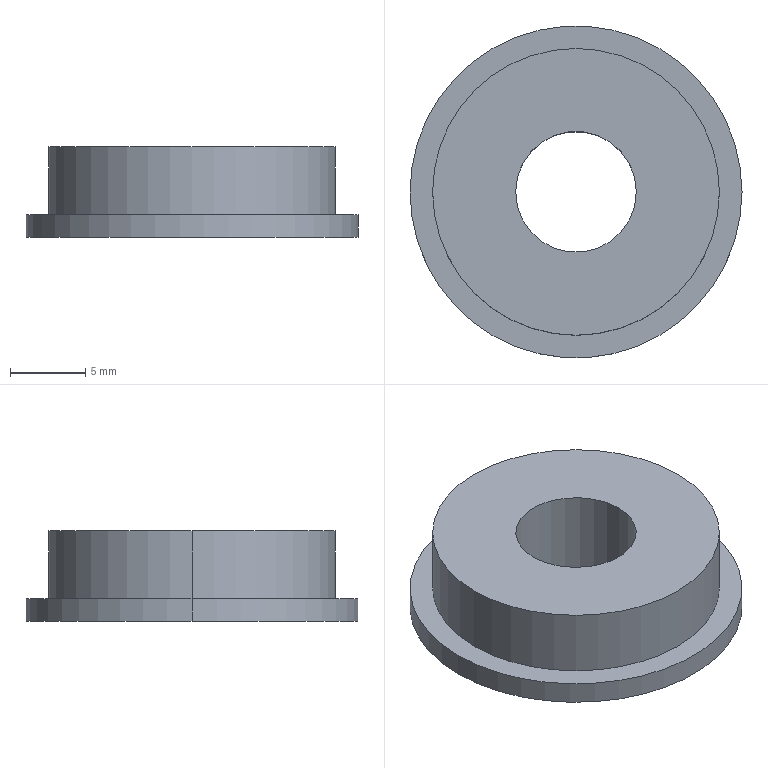Part | NX | 1 solid | 9 faces | box 22 x 22 x 6 mm | volume 1544 mm3 | cylinder 6 | plane 3 | commonest cylinder face diameters 8 x2 19 x2 22 x2
STEP:
#1=CARTESIAN_POINT('',(655.81,171.903,-33.25));
#2=VERTEX_POINT('',#1);
#3=CARTESIAN_POINT('',(633.81,171.903,-33.25));
#4=VERTEX_POINT('',#3);
#5=CARTESIAN_POINT('',(644.81,171.903,-33.25));
#6=DIRECTION('',(0.,0.,1.));
#7=DIRECTION('',(1.,0.,0.));
#8=AXIS2_PLACEMENT_3D('',#5,#6,#7);
#9=CIRCLE('',#8,11.);
#10=EDGE_CURVE('',#2,#4,#9,.T.);
#11=ORIENTED_EDGE('',*,*,#10,.T.);
#12=CARTESIAN_POINT('',(633.81,171.903,-31.75));
#13=VERTEX_POINT('',#12);
#14=CARTESIAN_POINT('',(633.81,171.903,-33.25));
#15=DIRECTION('',(0.,0.,1.));
#16=VECTOR('',#15,1000.);
#17=LINE('',#14,#16);
#18=EDGE_CURVE('',#4,#13,#17,.T.);
#19=ORIENTED_EDGE('',*,*,#18,.T.);
#20=CARTESIAN_POINT('',(655.81,171.903,-31.75));
#21=VERTEX_POINT('',#20);
#22=CARTESIAN_POINT('',(644.81,171.903,-31.75));
#23=DIRECTION('',(0.,0.,1.));
#24=DIRECTION('',(1.,0.,0.));
#25=AXIS2_PLACEMENT_3D('',#22,#23,#24);
#26=CIRCLE('',#25,11.);
#27=EDGE_CURVE('',#21,#13,#26,.T.);
#28=ORIENTED_EDGE('',*,*,#27,.F.);
#29=CARTESIAN_POINT('',(655.81,171.903,-33.25));
#30=DIRECTION('',(0.,0.,1.));
#31=VECTOR('',#30,1000.);
#32=LINE('',#29,#31);
#33=EDGE_CURVE('',#2,#21,#32,.T.);
#34=ORIENTED_EDGE('',*,*,#33,.F.);
#35=EDGE_LOOP('',(#11,#19,#28,#34));
#36=FACE_BOUND('',#35,.T.);
#37=CARTESIAN_POINT('',(644.81,171.903,-33.25));
#38=DIRECTION('',(0.,0.,1.));
#39=DIRECTION('',(1.,0.,0.));
#40=AXIS2_PLACEMENT_3D('',#37,#38,#39);
#41=CYLINDRICAL_SURFACE('',#40,11.);
#42=ADVANCED_FACE('',(#36),#41,.T.);
#43=ORIENTED_EDGE('',*,*,#10,.F.);
#44=CARTESIAN_POINT('',(644.81,171.903,-33.25));
#45=DIRECTION('',(0.,0.,1.));
#46=DIRECTION('',(1.,0.,0.));
#47=AXIS2_PLACEMENT_3D('',#44,#45,#46);
#48=CIRCLE('',#47,11.);
#49=EDGE_CURVE('',#4,#2,#48,.T.);
#50=ORIENTED_EDGE('',*,*,#49,.F.);
#51=EDGE_LOOP('',(#43,#50));
#52=FACE_BOUND('',#51,.T.);
#53=CARTESIAN_POINT('',(640.81,171.903,-33.25));
#54=VERTEX_POINT('',#53);
#55=CARTESIAN_POINT('',(648.81,171.903,-33.25));
#56=VERTEX_POINT('',#55);
#57=CARTESIAN_POINT('',(644.81,171.903,-33.25));
#58=DIRECTION('',(0.,0.,1.));
#59=DIRECTION('',(1.,0.,0.));
#60=AXIS2_PLACEMENT_3D('',#57,#58,#59);
#61=CIRCLE('',#60,4.);
#62=EDGE_CURVE('',#54,#56,#61,.T.);
#63=ORIENTED_EDGE('',*,*,#62,.T.);
#64=CARTESIAN_POINT('',(644.81,171.903,-33.25));
#65=DIRECTION('',(0.,0.,1.));
#66=DIRECTION('',(1.,0.,0.));
#67=AXIS2_PLACEMENT_3D('',#64,#65,#66);
#68=CIRCLE('',#67,4.);
#69=EDGE_CURVE('',#56,#54,#68,.T.);
#70=ORIENTED_EDGE('',*,*,#69,.T.);
#71=EDGE_LOOP('',(#63,#70));
#72=FACE_BOUND('',#71,.T.);
#73=CARTESIAN_POINT('',(647.81,186.903,-33.25));
#74=DIRECTION('',(0.,0.,1.));
#75=DIRECTION('',(1.,0.,0.));
#76=AXIS2_PLACEMENT_3D('',#73,#74,#75);
#77=PLANE('',#76);
#78=ADVANCED_FACE('',(#52,#72),#77,.F.);
#79=ORIENTED_EDGE('',*,*,#27,.T.);
#80=CARTESIAN_POINT('',(644.81,171.903,-31.75));
#81=DIRECTION('',(0.,0.,1.));
#82=DIRECTION('',(1.,0.,0.));
#83=AXIS2_PLACEMENT_3D('',#80,#81,#82);
#84=CIRCLE('',#83,11.);
#85=EDGE_CURVE('',#13,#21,#84,.T.);
#86=ORIENTED_EDGE('',*,*,#85,.T.);
#87=EDGE_LOOP('',(#79,#86));
#88=FACE_BOUND('',#87,.T.);
#89=CARTESIAN_POINT('',(654.31,171.903,-31.75));
#90=VERTEX_POINT('',#89);
#91=CARTESIAN_POINT('',(635.31,171.903,-31.75));
#92=VERTEX_POINT('',#91);
#93=CARTESIAN_POINT('',(644.81,171.903,-31.75));
#94=DIRECTION('',(0.,0.,1.));
#95=DIRECTION('',(1.,0.,0.));
#96=AXIS2_PLACEMENT_3D('',#93,#94,#95);
#97=CIRCLE('',#96,9.5);
#98=EDGE_CURVE('',#90,#92,#97,.T.);
#99=ORIENTED_EDGE('',*,*,#98,.F.);
#100=CARTESIAN_POINT('',(644.81,171.903,-31.75));
#101=DIRECTION('',(0.,0.,1.));
#102=DIRECTION('',(1.,0.,0.));
#103=AXIS2_PLACEMENT_3D('',#100,#101,#102);
#104=CIRCLE('',#103,9.5);
#105=EDGE_CURVE('',#92,#90,#104,.T.);
#106=ORIENTED_EDGE('',*,*,#105,.F.);
#107=EDGE_LOOP('',(#99,#106));
#108=FACE_BOUND('',#107,.T.);
#109=CARTESIAN_POINT('',(647.81,186.903,-31.75));
#110=DIRECTION('',(0.,0.,1.));
#111=DIRECTION('',(1.,0.,0.));
#112=AXIS2_PLACEMENT_3D('',#109,#110,#111);
#113=PLANE('',#112);
#114=ADVANCED_FACE('',(#88,#108),#113,.T.);
#115=CARTESIAN_POINT('',(654.31,171.903,-27.25));
#116=VERTEX_POINT('',#115);
#117=CARTESIAN_POINT('',(635.31,171.903,-27.25));
#118=VERTEX_POINT('',#117);
#119=CARTESIAN_POINT('',(644.81,171.903,-27.25));
#120=DIRECTION('',(0.,0.,1.));
#121=DIRECTION('',(1.,0.,0.));
#122=AXIS2_PLACEMENT_3D('',#119,#120,#121);
#123=CIRCLE('',#122,9.5);
#124=EDGE_CURVE('',#116,#118,#123,.T.);
#125=ORIENTED_EDGE('',*,*,#124,.F.);
#126=CARTESIAN_POINT('',(654.31,171.903,-31.75));
#127=DIRECTION('',(0.,0.,1.));
#128=VECTOR('',#127,1000.);
#129=LINE('',#126,#128);
#130=EDGE_CURVE('',#90,#116,#129,.T.);
#131=ORIENTED_EDGE('',*,*,#130,.F.);
#132=ORIENTED_EDGE('',*,*,#98,.T.);
#133=CARTESIAN_POINT('',(635.31,171.903,-31.75));
#134=DIRECTION('',(0.,0.,1.));
#135=VECTOR('',#134,1000.);
#136=LINE('',#133,#135);
#137=EDGE_CURVE('',#92,#118,#136,.T.);
#138=ORIENTED_EDGE('',*,*,#137,.T.);
#139=EDGE_LOOP('',(#125,#131,#132,#138));
#140=FACE_BOUND('',#139,.T.);
#141=CARTESIAN_POINT('',(644.81,171.903,-31.75));
#142=DIRECTION('',(0.,0.,1.));
#143=DIRECTION('',(1.,0.,0.));
#144=AXIS2_PLACEMENT_3D('',#141,#142,#143);
#145=CYLINDRICAL_SURFACE('',#144,9.5);
#146=ADVANCED_FACE('',(#140),#145,.T.);
#147=ORIENTED_EDGE('',*,*,#124,.T.);
#148=CARTESIAN_POINT('',(644.81,171.903,-27.25));
#149=DIRECTION('',(0.,0.,1.));
#150=DIRECTION('',(1.,0.,0.));
#151=AXIS2_PLACEMENT_3D('',#148,#149,#150);
#152=CIRCLE('',#151,9.5);
#153=EDGE_CURVE('',#118,#116,#152,.T.);
#154=ORIENTED_EDGE('',*,*,#153,.T.);
#155=EDGE_LOOP('',(#147,#154));
#156=FACE_BOUND('',#155,.T.);
#157=CARTESIAN_POINT('',(640.81,171.903,-27.25));
#158=VERTEX_POINT('',#157);
#159=CARTESIAN_POINT('',(648.81,171.903,-27.25));
#160=VERTEX_POINT('',#159);
#161=CARTESIAN_POINT('',(644.81,171.903,-27.25));
#162=DIRECTION('',(0.,0.,1.));
#163=DIRECTION('',(1.,0.,0.));
#164=AXIS2_PLACEMENT_3D('',#161,#162,#163);
#165=CIRCLE('',#164,4.);
#166=EDGE_CURVE('',#158,#160,#165,.T.);
#167=ORIENTED_EDGE('',*,*,#166,.F.);
#168=CARTESIAN_POINT('',(644.81,171.903,-27.25));
#169=DIRECTION('',(0.,0.,1.));
#170=DIRECTION('',(1.,0.,0.));
#171=AXIS2_PLACEMENT_3D('',#168,#169,#170);
#172=CIRCLE('',#171,4.);
#173=EDGE_CURVE('',#160,#158,#172,.T.);
#174=ORIENTED_EDGE('',*,*,#173,.F.);
#175=EDGE_LOOP('',(#167,#174));
#176=FACE_BOUND('',#175,.T.);
#177=CARTESIAN_POINT('',(646.88,172.371,-27.25));
#178=DIRECTION('',(0.,0.,1.));
#179=DIRECTION('',(1.,0.,0.));
#180=AXIS2_PLACEMENT_3D('',#177,#178,#179);
#181=PLANE('',#180);
#182=ADVANCED_FACE('',(#156,#176),#181,.T.);
#183=ORIENTED_EDGE('',*,*,#62,.F.);
#184=CARTESIAN_POINT('',(640.81,171.903,-33.85));
#185=DIRECTION('',(0.,0.,1.));
#186=VECTOR('',#185,1000.);
#187=LINE('',#184,#186);
#188=EDGE_CURVE('',#54,#158,#187,.T.);
#189=ORIENTED_EDGE('',*,*,#188,.T.);
#190=ORIENTED_EDGE('',*,*,#166,.T.);
#191=CARTESIAN_POINT('',(648.81,171.903,-33.85));
#192=DIRECTION('',(0.,0.,1.));
#193=VECTOR('',#192,1000.);
#194=LINE('',#191,#193);
#195=EDGE_CURVE('',#56,#160,#194,.T.);
#196=ORIENTED_EDGE('',*,*,#195,.F.);
#197=EDGE_LOOP('',(#183,#189,#190,#196));
#198=FACE_BOUND('',#197,.T.);
#199=CARTESIAN_POINT('',(644.81,171.903,-33.85));
#200=DIRECTION('',(0.,0.,1.));
#201=DIRECTION('',(1.,0.,0.));
#202=AXIS2_PLACEMENT_3D('',#199,#200,#201);
#203=CYLINDRICAL_SURFACE('',#202,4.);
#204=ADVANCED_FACE('',(#198),#203,.F.);
#205=ORIENTED_EDGE('',*,*,#33,.T.);
#206=ORIENTED_EDGE('',*,*,#85,.F.);
#207=ORIENTED_EDGE('',*,*,#18,.F.);
#208=ORIENTED_EDGE('',*,*,#49,.T.);
#209=EDGE_LOOP('',(#205,#206,#207,#208));
#210=FACE_BOUND('',#209,.T.);
#211=CARTESIAN_POINT('',(644.81,171.903,-33.25));
#212=DIRECTION('',(0.,0.,1.));
#213=DIRECTION('',(1.,0.,0.));
#214=AXIS2_PLACEMENT_3D('',#211,#212,#213);
#215=CYLINDRICAL_SURFACE('',#214,11.);
#216=ADVANCED_FACE('',(#210),#215,.T.);
#217=ORIENTED_EDGE('',*,*,#130,.T.);
#218=ORIENTED_EDGE('',*,*,#153,.F.);
#219=ORIENTED_EDGE('',*,*,#137,.F.);
#220=ORIENTED_EDGE('',*,*,#105,.T.);
#221=EDGE_LOOP('',(#217,#218,#219,#220));
#222=FACE_BOUND('',#221,.T.);
#223=CARTESIAN_POINT('',(644.81,171.903,-31.75));
#224=DIRECTION('',(0.,0.,1.));
#225=DIRECTION('',(1.,0.,0.));
#226=AXIS2_PLACEMENT_3D('',#223,#224,#225);
#227=CYLINDRICAL_SURFACE('',#226,9.5);
#228=ADVANCED_FACE('',(#222),#227,.T.);
#229=ORIENTED_EDGE('',*,*,#195,.T.);
#230=ORIENTED_EDGE('',*,*,#173,.T.);
#231=ORIENTED_EDGE('',*,*,#188,.F.);
#232=ORIENTED_EDGE('',*,*,#69,.F.);
#233=EDGE_LOOP('',(#229,#230,#231,#232));
#234=FACE_BOUND('',#233,.T.);
#235=CARTESIAN_POINT('',(644.81,171.903,-33.85));
#236=DIRECTION('',(0.,0.,1.));
#237=DIRECTION('',(1.,0.,0.));
#238=AXIS2_PLACEMENT_3D('',#235,#236,#237);
#239=CYLINDRICAL_SURFACE('',#238,4.);
#240=ADVANCED_FACE('',(#234),#239,.F.);
#241=CLOSED_SHELL('',(#42,#78,#114,#146,#182,#204,#216,#228,#240));
#242=MANIFOLD_SOLID_BREP('',#241);
#243=(LENGTH_UNIT()NAMED_UNIT(*)SI_UNIT(.MILLI.,.METRE.));
#244=UNCERTAINTY_MEASURE_WITH_UNIT(LENGTH_MEASURE(0.00001),#243,'','');
#245=(NAMED_UNIT(*)PLANE_ANGLE_UNIT()SI_UNIT($,.RADIAN.));
#246=(NAMED_UNIT(*)SI_UNIT($,.STERADIAN.)SOLID_ANGLE_UNIT());
#247=(GEOMETRIC_REPRESENTATION_CONTEXT(3)GLOBAL_UNCERTAINTY_ASSIGNED_CONTEXT((#244))GLOBAL_UNIT_ASSIGNED_CONTEXT((#243,#245,#246))REPRESENTATION_CONTEXT('',''));
#248=ADVANCED_BREP_SHAPE_REPRESENTATION('',(#242),#247);